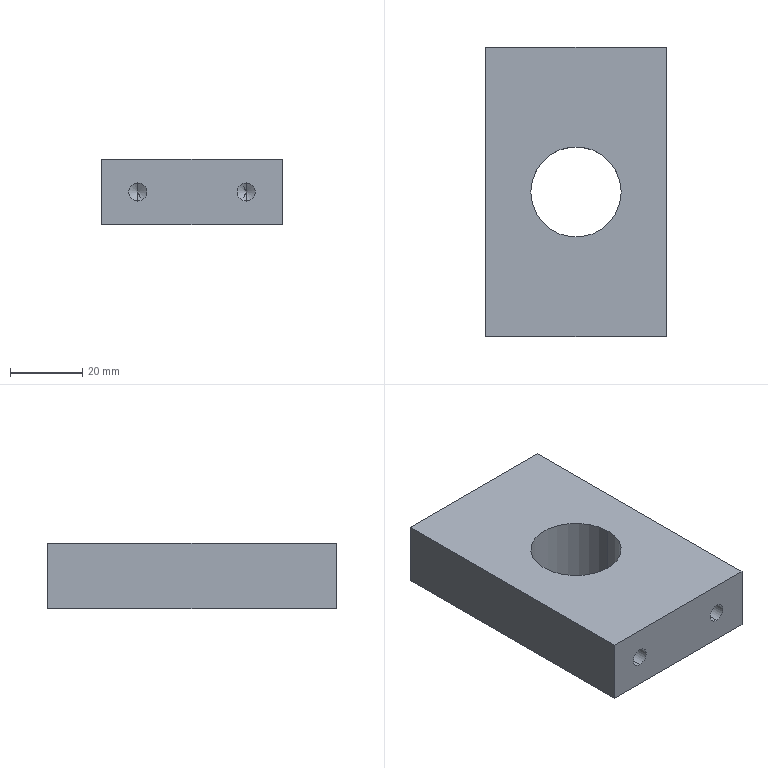Part | STEP file | BU-A03a | 1 solid | 24 faces | box 50 x 80 x 18 mm | volume 61790 mm3 | cylinder 10 | cone 8 | plane 6 | commonest cylinder face diameters 5 x8 25 x2